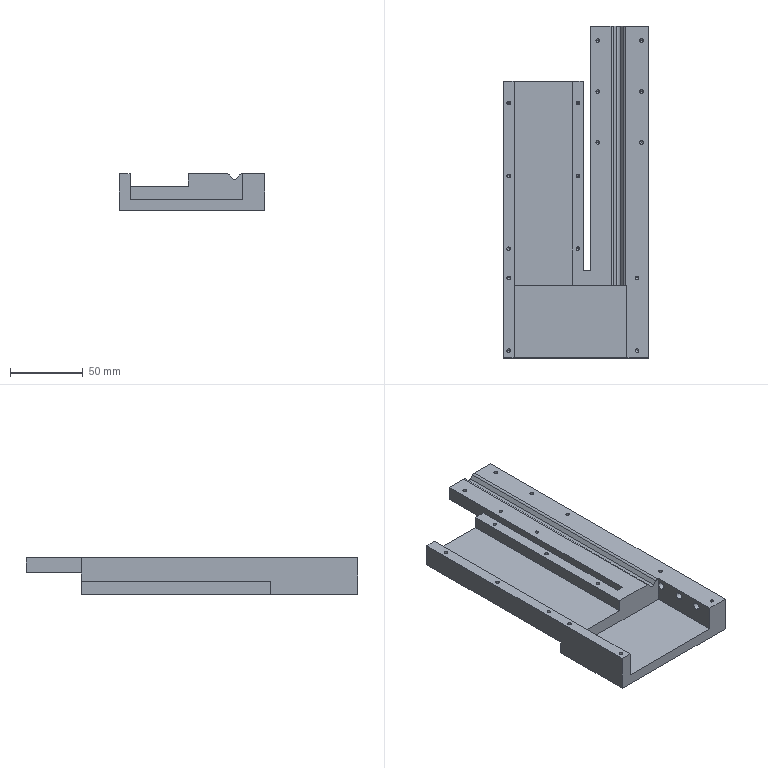Part | SolidWorks | features ICE 8, HoleWzd 3, Extrusion 1, Fillet 1, MoveFace 1 | 1 solid | 109 faces | box 100 x 228 x 25 mm | volume 243999 mm3 | cylinder 47 | cone 32 | plane 30 | commonest cylinder face diameters 2.5 x38 5.105 x6 4 x3